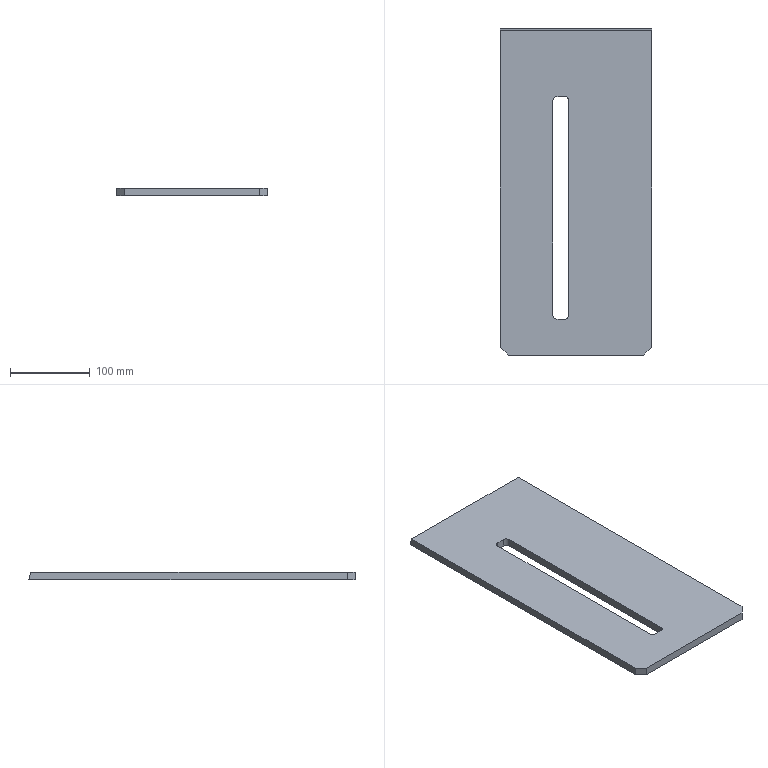Part | STEP file | 001-003-Shaft storage cylinder mounting plate | 1 solid | 16 faces | box 190 x 410.5 x 10 mm | volume 720796 mm3 | plane 12 | cylinder 4 | commonest cylinder face diameters 10 x4
STEP:
#1=CARTESIAN_POINT('',(0.,0.,0.));
#2=DIRECTION('',(0.,0.,1.));
#3=DIRECTION('',(1.,0.,0.));
#4=AXIS2_PLACEMENT_3D('',#1,#2,#3);
#5=CARTESIAN_POINT('',(95.,-195.25,10.));
#6=VERTEX_POINT('',#5);
#7=CARTESIAN_POINT('',(95.,202.757,10.));
#8=VERTEX_POINT('',#7);
#9=CARTESIAN_POINT('',(95.,-205.25,10.));
#10=DIRECTION('',(0.,1.,0.));
#11=VECTOR('',#10,1.);
#12=LINE('',#9,#11);
#13=CARTESIAN_POINT('',(95.,-205.25,10.));
#14=DIRECTION('',(-1.,0.,0.));
#15=DIRECTION('',(0.,0.,1.));
#16=AXIS2_PLACEMENT_3D('',#13,#14,#15);
#17=PLANE('',#16);
#18=CARTESIAN_POINT('',(0.,0.));
#19=DIRECTION('',(0.,1.));
#20=VECTOR('',#19,1.);
#21=LINE('',#18,#20);
#22=(GEOMETRIC_REPRESENTATION_CONTEXT(2)PARAMETRIC_REPRESENTATION_CONTEXT()REPRESENTATION_CONTEXT('',''));
#23=DEFINITIONAL_REPRESENTATION('',(#21),#22);
#24=PCURVE('',#17,#23);
#25=CARTESIAN_POINT('',(0.,0.,10.));
#26=DIRECTION('',(0.,0.,-1.));
#27=DIRECTION('',(-1.,0.,0.));
#28=AXIS2_PLACEMENT_3D('',#25,#26,#27);
#29=PLANE('',#28);
#30=CARTESIAN_POINT('',(-95.,-205.25));
#31=DIRECTION('',(0.,1.));
#32=VECTOR('',#31,1.);
#33=LINE('',#30,#32);
#34=(GEOMETRIC_REPRESENTATION_CONTEXT(2)PARAMETRIC_REPRESENTATION_CONTEXT()REPRESENTATION_CONTEXT('',''));
#35=DEFINITIONAL_REPRESENTATION('',(#33),#34);
#36=PCURVE('',#29,#35);
#37=SURFACE_CURVE('',#12,(#24,#36),.PCURVE_S1.);
#38=EDGE_CURVE('',#6,#8,#37,.T.);
#39=ORIENTED_EDGE('',*,*,#38,.F.);
#40=CARTESIAN_POINT('',(95.,-195.25,0.));
#41=VERTEX_POINT('',#40);
#42=CARTESIAN_POINT('',(95.,-195.25,10.));
#43=DIRECTION('',(0.,0.,-1.));
#44=VECTOR('',#43,1.);
#45=LINE('',#42,#44);
#46=CARTESIAN_POINT('',(0.,10.));
#47=DIRECTION('',(-1.,0.));
#48=VECTOR('',#47,1.);
#49=LINE('',#46,#48);
#50=(GEOMETRIC_REPRESENTATION_CONTEXT(2)PARAMETRIC_REPRESENTATION_CONTEXT()REPRESENTATION_CONTEXT('',''));
#51=DEFINITIONAL_REPRESENTATION('',(#49),#50);
#52=PCURVE('',#17,#51);
#53=CARTESIAN_POINT('',(95.,-195.25,10.));
#54=DIRECTION('',(-0.7071,0.7071,0.));
#55=DIRECTION('',(0.,0.,-1.));
#56=AXIS2_PLACEMENT_3D('',#53,#54,#55);
#57=PLANE('',#56);
#58=CARTESIAN_POINT('',(0.,0.));
#59=DIRECTION('',(1.,0.));
#60=VECTOR('',#59,1.);
#61=LINE('',#58,#60);
#62=(GEOMETRIC_REPRESENTATION_CONTEXT(2)PARAMETRIC_REPRESENTATION_CONTEXT()REPRESENTATION_CONTEXT('',''));
#63=DEFINITIONAL_REPRESENTATION('',(#61),#62);
#64=PCURVE('',#57,#63);
#65=SURFACE_CURVE('',#45,(#52,#64),.PCURVE_S1.);
#66=EDGE_CURVE('',#6,#41,#65,.T.);
#67=ORIENTED_EDGE('',*,*,#66,.T.);
#68=CARTESIAN_POINT('',(95.,205.25,0.));
#69=VERTEX_POINT('',#68);
#70=CARTESIAN_POINT('',(95.,-205.25,0.));
#71=DIRECTION('',(0.,1.,0.));
#72=VECTOR('',#71,1.);
#73=LINE('',#70,#72);
#74=CARTESIAN_POINT('',(-10.,0.));
#75=DIRECTION('',(0.,1.));
#76=VECTOR('',#75,1.);
#77=LINE('',#74,#76);
#78=(GEOMETRIC_REPRESENTATION_CONTEXT(2)PARAMETRIC_REPRESENTATION_CONTEXT()REPRESENTATION_CONTEXT('',''));
#79=DEFINITIONAL_REPRESENTATION('',(#77),#78);
#80=PCURVE('',#17,#79);
#81=CARTESIAN_POINT('',(0.,0.,0.));
#82=DIRECTION('',(0.,0.,-1.));
#83=DIRECTION('',(-1.,0.,0.));
#84=AXIS2_PLACEMENT_3D('',#81,#82,#83);
#85=PLANE('',#84);
#86=CARTESIAN_POINT('',(-95.,-205.25));
#87=DIRECTION('',(0.,1.));
#88=VECTOR('',#87,1.);
#89=LINE('',#86,#88);
#90=(GEOMETRIC_REPRESENTATION_CONTEXT(2)PARAMETRIC_REPRESENTATION_CONTEXT()REPRESENTATION_CONTEXT('',''));
#91=DEFINITIONAL_REPRESENTATION('',(#89),#90);
#92=PCURVE('',#85,#91);
#93=SURFACE_CURVE('',#73,(#80,#92),.PCURVE_S1.);
#94=EDGE_CURVE('',#41,#69,#93,.T.);
#95=ORIENTED_EDGE('',*,*,#94,.T.);
#96=CARTESIAN_POINT('',(95.,205.25,0.));
#97=DIRECTION('',(0.,0.2419,-0.9703));
#98=VECTOR('',#97,1.);
#99=LINE('',#96,#98);
#100=CARTESIAN_POINT('',(-10.,410.5));
#101=DIRECTION('',(-0.9703,0.2419));
#102=VECTOR('',#101,1.);
#103=LINE('',#100,#102);
#104=(GEOMETRIC_REPRESENTATION_CONTEXT(2)PARAMETRIC_REPRESENTATION_CONTEXT()REPRESENTATION_CONTEXT('',''));
#105=DEFINITIONAL_REPRESENTATION('',(#103),#104);
#106=PCURVE('',#17,#105);
#107=CARTESIAN_POINT('',(-95.,205.25,0.));
#108=DIRECTION('',(0.,-0.9703,-0.2419));
#109=DIRECTION('',(0.,0.2419,-0.9703));
#110=AXIS2_PLACEMENT_3D('',#107,#108,#109);
#111=PLANE('',#110);
#112=CARTESIAN_POINT('',(0.,190.));
#113=DIRECTION('',(1.,0.));
#114=VECTOR('',#113,1.);
#115=LINE('',#112,#114);
#116=(GEOMETRIC_REPRESENTATION_CONTEXT(2)PARAMETRIC_REPRESENTATION_CONTEXT()REPRESENTATION_CONTEXT('',''));
#117=DEFINITIONAL_REPRESENTATION('',(#115),#116);
#118=PCURVE('',#111,#117);
#119=SURFACE_CURVE('',#99,(#106,#118),.PCURVE_S1.);
#120=EDGE_CURVE('',#8,#69,#119,.T.);
#121=ORIENTED_EDGE('',*,*,#120,.F.);
#122=EDGE_LOOP('',(#39,#67,#95,#121));
#123=FACE_BOUND('',#122,.T.);
#124=ADVANCED_FACE('',(#123),#17,.F.);
#125=CARTESIAN_POINT('',(-95.,205.25,0.));
#126=VERTEX_POINT('',#125);
#127=CARTESIAN_POINT('',(-95.,-195.25,0.));
#128=VERTEX_POINT('',#127);
#129=CARTESIAN_POINT('',(-95.,-205.25,0.));
#130=DIRECTION('',(0.,-1.,0.));
#131=VECTOR('',#130,1.);
#132=LINE('',#129,#131);
#133=CARTESIAN_POINT('',(-95.,-205.25,10.));
#134=DIRECTION('',(1.,0.,0.));
#135=DIRECTION('',(0.,0.,-1.));
#136=AXIS2_PLACEMENT_3D('',#133,#134,#135);
#137=PLANE('',#136);
#138=CARTESIAN_POINT('',(10.,0.));
#139=DIRECTION('',(0.,-1.));
#140=VECTOR('',#139,1.);
#141=LINE('',#138,#140);
#142=(GEOMETRIC_REPRESENTATION_CONTEXT(2)PARAMETRIC_REPRESENTATION_CONTEXT()REPRESENTATION_CONTEXT('',''));
#143=DEFINITIONAL_REPRESENTATION('',(#141),#142);
#144=PCURVE('',#137,#143);
#145=CARTESIAN_POINT('',(95.,-205.25));
#146=DIRECTION('',(0.,-1.));
#147=VECTOR('',#146,1.);
#148=LINE('',#145,#147);
#149=(GEOMETRIC_REPRESENTATION_CONTEXT(2)PARAMETRIC_REPRESENTATION_CONTEXT()REPRESENTATION_CONTEXT('',''));
#150=DEFINITIONAL_REPRESENTATION('',(#148),#149);
#151=PCURVE('',#85,#150);
#152=SURFACE_CURVE('',#132,(#144,#151),.PCURVE_S1.);
#153=EDGE_CURVE('',#126,#128,#152,.T.);
#154=ORIENTED_EDGE('',*,*,#153,.T.);
#155=CARTESIAN_POINT('',(-95.,-195.25,10.));
#156=VERTEX_POINT('',#155);
#157=CARTESIAN_POINT('',(-95.,-195.25,10.));
#158=DIRECTION('',(0.,0.,1.));
#159=VECTOR('',#158,1.);
#160=LINE('',#157,#159);
#161=CARTESIAN_POINT('',(0.,10.));
#162=DIRECTION('',(-1.,0.));
#163=VECTOR('',#162,1.);
#164=LINE('',#161,#163);
#165=(GEOMETRIC_REPRESENTATION_CONTEXT(2)PARAMETRIC_REPRESENTATION_CONTEXT()REPRESENTATION_CONTEXT('',''));
#166=DEFINITIONAL_REPRESENTATION('',(#164),#165);
#167=PCURVE('',#137,#166);
#168=CARTESIAN_POINT('',(-85.,-205.25,10.));
#169=DIRECTION('',(0.7071,0.7071,0.));
#170=DIRECTION('',(0.,0.,-1.));
#171=AXIS2_PLACEMENT_3D('',#168,#169,#170);
#172=PLANE('',#171);
#173=CARTESIAN_POINT('',(0.,14.142));
#174=DIRECTION('',(-1.,0.));
#175=VECTOR('',#174,1.);
#176=LINE('',#173,#175);
#177=(GEOMETRIC_REPRESENTATION_CONTEXT(2)PARAMETRIC_REPRESENTATION_CONTEXT()REPRESENTATION_CONTEXT('',''));
#178=DEFINITIONAL_REPRESENTATION('',(#176),#177);
#179=PCURVE('',#172,#178);
#180=SURFACE_CURVE('',#160,(#167,#179),.PCURVE_S1.);
#181=EDGE_CURVE('',#128,#156,#180,.T.);
#182=ORIENTED_EDGE('',*,*,#181,.T.);
#183=CARTESIAN_POINT('',(-95.,202.757,10.));
#184=VERTEX_POINT('',#183);
#185=CARTESIAN_POINT('',(-95.,-205.25,10.));
#186=DIRECTION('',(0.,-1.,0.));
#187=VECTOR('',#186,1.);
#188=LINE('',#185,#187);
#189=CARTESIAN_POINT('',(0.,0.));
#190=DIRECTION('',(0.,-1.));
#191=VECTOR('',#190,1.);
#192=LINE('',#189,#191);
#193=(GEOMETRIC_REPRESENTATION_CONTEXT(2)PARAMETRIC_REPRESENTATION_CONTEXT()REPRESENTATION_CONTEXT('',''));
#194=DEFINITIONAL_REPRESENTATION('',(#192),#193);
#195=PCURVE('',#137,#194);
#196=CARTESIAN_POINT('',(95.,-205.25));
#197=DIRECTION('',(0.,-1.));
#198=VECTOR('',#197,1.);
#199=LINE('',#196,#198);
#200=(GEOMETRIC_REPRESENTATION_CONTEXT(2)PARAMETRIC_REPRESENTATION_CONTEXT()REPRESENTATION_CONTEXT('',''));
#201=DEFINITIONAL_REPRESENTATION('',(#199),#200);
#202=PCURVE('',#29,#201);
#203=SURFACE_CURVE('',#188,(#195,#202),.PCURVE_S1.);
#204=EDGE_CURVE('',#184,#156,#203,.T.);
#205=ORIENTED_EDGE('',*,*,#204,.F.);
#206=CARTESIAN_POINT('',(-95.,205.25,0.));
#207=DIRECTION('',(0.,0.2419,-0.9703));
#208=VECTOR('',#207,1.);
#209=LINE('',#206,#208);
#210=CARTESIAN_POINT('',(10.,410.5));
#211=DIRECTION('',(0.9703,0.2419));
#212=VECTOR('',#211,1.);
#213=LINE('',#210,#212);
#214=(GEOMETRIC_REPRESENTATION_CONTEXT(2)PARAMETRIC_REPRESENTATION_CONTEXT()REPRESENTATION_CONTEXT('',''));
#215=DEFINITIONAL_REPRESENTATION('',(#213),#214);
#216=PCURVE('',#137,#215);
#217=CARTESIAN_POINT('',(0.,0.));
#218=DIRECTION('',(1.,0.));
#219=VECTOR('',#218,1.);
#220=LINE('',#217,#219);
#221=(GEOMETRIC_REPRESENTATION_CONTEXT(2)PARAMETRIC_REPRESENTATION_CONTEXT()REPRESENTATION_CONTEXT('',''));
#222=DEFINITIONAL_REPRESENTATION('',(#220),#221);
#223=PCURVE('',#111,#222);
#224=SURFACE_CURVE('',#209,(#216,#223),.PCURVE_S1.);
#225=EDGE_CURVE('',#184,#126,#224,.T.);
#226=ORIENTED_EDGE('',*,*,#225,.T.);
#227=EDGE_LOOP('',(#154,#182,#205,#226));
#228=FACE_BOUND('',#227,.T.);
#229=ADVANCED_FACE('',(#228),#137,.F.);
#230=CARTESIAN_POINT('',(-85.,-205.25,0.));
#231=VERTEX_POINT('',#230);
#232=CARTESIAN_POINT('',(85.,-205.25,0.));
#233=VERTEX_POINT('',#232);
#234=CARTESIAN_POINT('',(-95.,-205.25,0.));
#235=DIRECTION('',(1.,0.,0.));
#236=VECTOR('',#235,1.);
#237=LINE('',#234,#236);
#238=CARTESIAN_POINT('',(-95.,-205.25,10.));
#239=DIRECTION('',(0.,1.,0.));
#240=DIRECTION('',(0.,0.,1.));
#241=AXIS2_PLACEMENT_3D('',#238,#239,#240);
#242=PLANE('',#241);
#243=CARTESIAN_POINT('',(-10.,0.));
#244=DIRECTION('',(0.,1.));
#245=VECTOR('',#244,1.);
#246=LINE('',#243,#245);
#247=(GEOMETRIC_REPRESENTATION_CONTEXT(2)PARAMETRIC_REPRESENTATION_CONTEXT()REPRESENTATION_CONTEXT('',''));
#248=DEFINITIONAL_REPRESENTATION('',(#246),#247);
#249=PCURVE('',#242,#248);
#250=CARTESIAN_POINT('',(95.,-205.25));
#251=DIRECTION('',(-1.,0.));
#252=VECTOR('',#251,1.);
#253=LINE('',#250,#252);
#254=(GEOMETRIC_REPRESENTATION_CONTEXT(2)PARAMETRIC_REPRESENTATION_CONTEXT()REPRESENTATION_CONTEXT('',''));
#255=DEFINITIONAL_REPRESENTATION('',(#253),#254);
#256=PCURVE('',#85,#255);
#257=SURFACE_CURVE('',#237,(#249,#256),.PCURVE_S1.);
#258=EDGE_CURVE('',#231,#233,#257,.T.);
#259=ORIENTED_EDGE('',*,*,#258,.T.);
#260=CARTESIAN_POINT('',(85.,-205.25,10.));
#261=VERTEX_POINT('',#260);
#262=CARTESIAN_POINT('',(85.,-205.25,10.));
#263=DIRECTION('',(0.,0.,1.));
#264=VECTOR('',#263,1.);
#265=LINE('',#262,#264);
#266=CARTESIAN_POINT('',(0.,180.));
#267=DIRECTION('',(1.,0.));
#268=VECTOR('',#267,1.);
#269=LINE('',#266,#268);
#270=(GEOMETRIC_REPRESENTATION_CONTEXT(2)PARAMETRIC_REPRESENTATION_CONTEXT()REPRESENTATION_CONTEXT('',''));
#271=DEFINITIONAL_REPRESENTATION('',(#269),#270);
#272=PCURVE('',#242,#271);
#273=CARTESIAN_POINT('',(0.,14.142));
#274=DIRECTION('',(-1.,0.));
#275=VECTOR('',#274,1.);
#276=LINE('',#273,#275);
#277=(GEOMETRIC_REPRESENTATION_CONTEXT(2)PARAMETRIC_REPRESENTATION_CONTEXT()REPRESENTATION_CONTEXT('',''));
#278=DEFINITIONAL_REPRESENTATION('',(#276),#277);
#279=PCURVE('',#57,#278);
#280=SURFACE_CURVE('',#265,(#272,#279),.PCURVE_S1.);
#281=EDGE_CURVE('',#233,#261,#280,.T.);
#282=ORIENTED_EDGE('',*,*,#281,.T.);
#283=CARTESIAN_POINT('',(-85.,-205.25,10.));
#284=VERTEX_POINT('',#283);
#285=CARTESIAN_POINT('',(-95.,-205.25,10.));
#286=DIRECTION('',(1.,0.,0.));
#287=VECTOR('',#286,1.);
#288=LINE('',#285,#287);
#289=CARTESIAN_POINT('',(0.,0.));
#290=DIRECTION('',(0.,1.));
#291=VECTOR('',#290,1.);
#292=LINE('',#289,#291);
#293=(GEOMETRIC_REPRESENTATION_CONTEXT(2)PARAMETRIC_REPRESENTATION_CONTEXT()REPRESENTATION_CONTEXT('',''));
#294=DEFINITIONAL_REPRESENTATION('',(#292),#293);
#295=PCURVE('',#242,#294);
#296=CARTESIAN_POINT('',(95.,-205.25));
#297=DIRECTION('',(-1.,0.));
#298=VECTOR('',#297,1.);
#299=LINE('',#296,#298);
#300=(GEOMETRIC_REPRESENTATION_CONTEXT(2)PARAMETRIC_REPRESENTATION_CONTEXT()REPRESENTATION_CONTEXT('',''));
#301=DEFINITIONAL_REPRESENTATION('',(#299),#300);
#302=PCURVE('',#29,#301);
#303=SURFACE_CURVE('',#288,(#295,#302),.PCURVE_S1.);
#304=EDGE_CURVE('',#284,#261,#303,.T.);
#305=ORIENTED_EDGE('',*,*,#304,.F.);
#306=CARTESIAN_POINT('',(-85.,-205.25,10.));
#307=DIRECTION('',(0.,0.,-1.));
#308=VECTOR('',#307,1.);
#309=LINE('',#306,#308);
#310=CARTESIAN_POINT('',(0.,10.));
#311=DIRECTION('',(-1.,0.));
#312=VECTOR('',#311,1.);
#313=LINE('',#310,#312);
#314=(GEOMETRIC_REPRESENTATION_CONTEXT(2)PARAMETRIC_REPRESENTATION_CONTEXT()REPRESENTATION_CONTEXT('',''));
#315=DEFINITIONAL_REPRESENTATION('',(#313),#314);
#316=PCURVE('',#242,#315);
#317=CARTESIAN_POINT('',(0.,0.));
#318=DIRECTION('',(1.,0.));
#319=VECTOR('',#318,1.);
#320=LINE('',#317,#319);
#321=(GEOMETRIC_REPRESENTATION_CONTEXT(2)PARAMETRIC_REPRESENTATION_CONTEXT()REPRESENTATION_CONTEXT('',''));
#322=DEFINITIONAL_REPRESENTATION('',(#320),#321);
#323=PCURVE('',#172,#322);
#324=SURFACE_CURVE('',#309,(#316,#323),.PCURVE_S1.);
#325=EDGE_CURVE('',#284,#231,#324,.T.);
#326=ORIENTED_EDGE('',*,*,#325,.T.);
#327=EDGE_LOOP('',(#259,#282,#305,#326));
#328=FACE_BOUND('',#327,.T.);
#329=ADVANCED_FACE('',(#328),#242,.F.);
#330=CARTESIAN_POINT('',(-14.,120.,10.));
#331=VERTEX_POINT('',#330);
#332=CARTESIAN_POINT('',(-24.,120.,10.));
#333=VERTEX_POINT('',#332);
#334=CARTESIAN_POINT('',(-9.,120.,10.));
#335=DIRECTION('',(-1.,0.,0.));
#336=VECTOR('',#335,1.);
#337=LINE('',#334,#336);
#338=CARTESIAN_POINT('',(9.,120.));
#339=DIRECTION('',(1.,0.));
#340=VECTOR('',#339,1.);
#341=LINE('',#338,#340);
#342=(GEOMETRIC_REPRESENTATION_CONTEXT(2)PARAMETRIC_REPRESENTATION_CONTEXT()REPRESENTATION_CONTEXT('',''));
#343=DEFINITIONAL_REPRESENTATION('',(#341),#342);
#344=PCURVE('',#29,#343);
#345=CARTESIAN_POINT('',(-9.,120.,0.));
#346=DIRECTION('',(0.,1.,0.));
#347=DIRECTION('',(0.,0.,1.));
#348=AXIS2_PLACEMENT_3D('',#345,#346,#347);
#349=PLANE('',#348);
#350=CARTESIAN_POINT('',(10.,0.));
#351=DIRECTION('',(0.,-1.));
#352=VECTOR('',#351,1.);
#353=LINE('',#350,#352);
#354=(GEOMETRIC_REPRESENTATION_CONTEXT(2)PARAMETRIC_REPRESENTATION_CONTEXT()REPRESENTATION_CONTEXT('',''));
#355=DEFINITIONAL_REPRESENTATION('',(#353),#354);
#356=PCURVE('',#349,#355);
#357=SURFACE_CURVE('',#337,(#344,#356),.PCURVE_S1.);
#358=EDGE_CURVE('',#331,#333,#357,.T.);
#359=ORIENTED_EDGE('',*,*,#358,.F.);
#360=CARTESIAN_POINT('',(-9.,115.,10.));
#361=VERTEX_POINT('',#360);
#362=CARTESIAN_POINT('',(-14.,115.,10.));
#363=DIRECTION('',(0.,0.,-1.));
#364=DIRECTION('',(-1.,0.,0.));
#365=AXIS2_PLACEMENT_3D('',#362,#363,#364);
#366=CIRCLE('',#365,5.);
#367=CARTESIAN_POINT('',(14.,115.));
#368=DIRECTION('',(1.,0.));
#369=AXIS2_PLACEMENT_2D('',#367,#368);
#370=CIRCLE('',#369,5.);
#371=(GEOMETRIC_REPRESENTATION_CONTEXT(2)PARAMETRIC_REPRESENTATION_CONTEXT()REPRESENTATION_CONTEXT('',''));
#372=DEFINITIONAL_REPRESENTATION('',(#370),#371);
#373=PCURVE('',#29,#372);
#374=CARTESIAN_POINT('',(-14.,115.,0.));
#375=DIRECTION('',(0.,0.,-1.));
#376=DIRECTION('',(-1.,0.,0.));
#377=AXIS2_PLACEMENT_3D('',#374,#375,#376);
#378=CYLINDRICAL_SURFACE('',#377,5.);
#379=CARTESIAN_POINT('',(0.,-10.));
#380=DIRECTION('',(1.,0.));
#381=VECTOR('',#380,1.);
#382=LINE('',#379,#381);
#383=(GEOMETRIC_REPRESENTATION_CONTEXT(2)PARAMETRIC_REPRESENTATION_CONTEXT()REPRESENTATION_CONTEXT('',''));
#384=DEFINITIONAL_REPRESENTATION('',(#382),#383);
#385=PCURVE('',#378,#384);
#386=SURFACE_CURVE('',#366,(#373,#385),.PCURVE_S1.);
#387=EDGE_CURVE('',#331,#361,#386,.T.);
#388=ORIENTED_EDGE('',*,*,#387,.T.);
#389=CARTESIAN_POINT('',(-9.,-155.,10.));
#390=VERTEX_POINT('',#389);
#391=CARTESIAN_POINT('',(-9.,-160.,10.));
#392=DIRECTION('',(0.,1.,0.));
#393=VECTOR('',#392,1.);
#394=LINE('',#391,#393);
#395=CARTESIAN_POINT('',(9.,-160.));
#396=DIRECTION('',(0.,1.));
#397=VECTOR('',#396,1.);
#398=LINE('',#395,#397);
#399=(GEOMETRIC_REPRESENTATION_CONTEXT(2)PARAMETRIC_REPRESENTATION_CONTEXT()REPRESENTATION_CONTEXT('',''));
#400=DEFINITIONAL_REPRESENTATION('',(#398),#399);
#401=PCURVE('',#29,#400);
#402=CARTESIAN_POINT('',(-9.,-160.,0.));
#403=DIRECTION('',(1.,0.,0.));
#404=DIRECTION('',(0.,0.,-1.));
#405=AXIS2_PLACEMENT_3D('',#402,#403,#404);
#406=PLANE('',#405);
#407=CARTESIAN_POINT('',(-10.,0.));
#408=DIRECTION('',(0.,1.));
#409=VECTOR('',#408,1.);
#410=LINE('',#407,#409);
#411=(GEOMETRIC_REPRESENTATION_CONTEXT(2)PARAMETRIC_REPRESENTATION_CONTEXT()REPRESENTATION_CONTEXT('',''));
#412=DEFINITIONAL_REPRESENTATION('',(#410),#411);
#413=PCURVE('',#406,#412);
#414=SURFACE_CURVE('',#394,(#401,#413),.PCURVE_S1.);
#415=EDGE_CURVE('',#390,#361,#414,.T.);
#416=ORIENTED_EDGE('',*,*,#415,.F.);
#417=CARTESIAN_POINT('',(-14.,-160.,10.));
#418=VERTEX_POINT('',#417);
#419=CARTESIAN_POINT('',(-14.,-155.,10.));
#420=DIRECTION('',(0.,0.,-1.));
#421=DIRECTION('',(-1.,0.,0.));
#422=AXIS2_PLACEMENT_3D('',#419,#420,#421);
#423=CIRCLE('',#422,5.);
#424=CARTESIAN_POINT('',(14.,-155.));
#425=DIRECTION('',(1.,0.));
#426=AXIS2_PLACEMENT_2D('',#424,#425);
#427=CIRCLE('',#426,5.);
#428=(GEOMETRIC_REPRESENTATION_CONTEXT(2)PARAMETRIC_REPRESENTATION_CONTEXT()REPRESENTATION_CONTEXT('',''));
#429=DEFINITIONAL_REPRESENTATION('',(#427),#428);
#430=PCURVE('',#29,#429);
#431=CARTESIAN_POINT('',(-14.,-155.,0.));
#432=DIRECTION('',(0.,0.,-1.));
#433=DIRECTION('',(-1.,0.,0.));
#434=AXIS2_PLACEMENT_3D('',#431,#432,#433);
#435=CYLINDRICAL_SURFACE('',#434,5.);
#436=CARTESIAN_POINT('',(0.,-10.));
#437=DIRECTION('',(1.,0.));
#438=VECTOR('',#437,1.);
#439=LINE('',#436,#438);
#440=(GEOMETRIC_REPRESENTATION_CONTEXT(2)PARAMETRIC_REPRESENTATION_CONTEXT()REPRESENTATION_CONTEXT('',''));
#441=DEFINITIONAL_REPRESENTATION('',(#439),#440);
#442=PCURVE('',#435,#441);
#443=SURFACE_CURVE('',#423,(#430,#442),.PCURVE_S1.);
#444=EDGE_CURVE('',#390,#418,#443,.T.);
#445=ORIENTED_EDGE('',*,*,#444,.T.);
#446=CARTESIAN_POINT('',(-24.,-160.,10.));
#447=VERTEX_POINT('',#446);
#448=CARTESIAN_POINT('',(-9.,-160.,10.));
#449=DIRECTION('',(1.,0.,0.));
#450=VECTOR('',#449,1.);
#451=LINE('',#448,#450);
#452=CARTESIAN_POINT('',(9.,-160.));
#453=DIRECTION('',(-1.,0.));
#454=VECTOR('',#453,1.);
#455=LINE('',#452,#454);
#456=(GEOMETRIC_REPRESENTATION_CONTEXT(2)PARAMETRIC_REPRESENTATION_CONTEXT()REPRESENTATION_CONTEXT('',''));
#457=DEFINITIONAL_REPRESENTATION('',(#455),#456);
#458=PCURVE('',#29,#457);
#459=CARTESIAN_POINT('',(-9.,-160.,0.));
#460=DIRECTION('',(0.,-1.,0.));
#461=DIRECTION('',(1.,0.,0.));
#462=AXIS2_PLACEMENT_3D('',#459,#460,#461);
#463=PLANE('',#462);
#464=CARTESIAN_POINT('',(0.,10.));
#465=DIRECTION('',(1.,0.));
#466=VECTOR('',#465,1.);
#467=LINE('',#464,#466);
#468=(GEOMETRIC_REPRESENTATION_CONTEXT(2)PARAMETRIC_REPRESENTATION_CONTEXT()REPRESENTATION_CONTEXT('',''));
#469=DEFINITIONAL_REPRESENTATION('',(#467),#468);
#470=PCURVE('',#463,#469);
#471=SURFACE_CURVE('',#451,(#458,#470),.PCURVE_S1.);
#472=EDGE_CURVE('',#447,#418,#471,.T.);
#473=ORIENTED_EDGE('',*,*,#472,.F.);
#474=CARTESIAN_POINT('',(-29.,-155.,10.));
#475=VERTEX_POINT('',#474);
#476=CARTESIAN_POINT('',(-24.,-155.,10.));
#477=DIRECTION('',(0.,0.,-1.));
#478=DIRECTION('',(-1.,0.,0.));
#479=AXIS2_PLACEMENT_3D('',#476,#477,#478);
#480=CIRCLE('',#479,5.);
#481=CARTESIAN_POINT('',(24.,-155.));
#482=DIRECTION('',(1.,0.));
#483=AXIS2_PLACEMENT_2D('',#481,#482);
#484=CIRCLE('',#483,5.);
#485=(GEOMETRIC_REPRESENTATION_CONTEXT(2)PARAMETRIC_REPRESENTATION_CONTEXT()REPRESENTATION_CONTEXT('',''));
#486=DEFINITIONAL_REPRESENTATION('',(#484),#485);
#487=PCURVE('',#29,#486);
#488=CARTESIAN_POINT('',(-24.,-155.,0.));
#489=DIRECTION('',(0.,0.,-1.));
#490=DIRECTION('',(-1.,0.,0.));
#491=AXIS2_PLACEMENT_3D('',#488,#489,#490);
#492=CYLINDRICAL_SURFACE('',#491,5.);
#493=CARTESIAN_POINT('',(0.,-10.));
#494=DIRECTION('',(1.,0.));
#495=VECTOR('',#494,1.);
#496=LINE('',#493,#495);
#497=(GEOMETRIC_REPRESENTATION_CONTEXT(2)PARAMETRIC_REPRESENTATION_CONTEXT()REPRESENTATION_CONTEXT('',''));
#498=DEFINITIONAL_REPRESENTATION('',(#496),#497);
#499=PCURVE('',#492,#498);
#500=SURFACE_CURVE('',#480,(#487,#499),.PCURVE_S1.);
#501=EDGE_CURVE('',#447,#475,#500,.T.);
#502=ORIENTED_EDGE('',*,*,#501,.T.);
#503=CARTESIAN_POINT('',(-29.,115.,10.));
#504=VERTEX_POINT('',#503);
#505=CARTESIAN_POINT('',(-29.,-160.,10.));
#506=DIRECTION('',(0.,-1.,0.));
#507=VECTOR('',#506,1.);
#508=LINE('',#505,#507);
#509=CARTESIAN_POINT('',(29.,-160.));
#510=DIRECTION('',(0.,-1.));
#511=VECTOR('',#510,1.);
#512=LINE('',#509,#511);
#513=(GEOMETRIC_REPRESENTATION_CONTEXT(2)PARAMETRIC_REPRESENTATION_CONTEXT()REPRESENTATION_CONTEXT('',''));
#514=DEFINITIONAL_REPRESENTATION('',(#512),#513);
#515=PCURVE('',#29,#514);
#516=CARTESIAN_POINT('',(-29.,-160.,0.));
#517=DIRECTION('',(-1.,0.,0.));
#518=DIRECTION('',(0.,-1.,0.));
#519=AXIS2_PLACEMENT_3D('',#516,#517,#518);
#520=PLANE('',#519);
#521=CARTESIAN_POINT('',(0.,10.));
#522=DIRECTION('',(1.,0.));
#523=VECTOR('',#522,1.);
#524=LINE('',#521,#523);
#525=(GEOMETRIC_REPRESENTATION_CONTEXT(2)PARAMETRIC_REPRESENTATION_CONTEXT()REPRESENTATION_CONTEXT('',''));
#526=DEFINITIONAL_REPRESENTATION('',(#524),#525);
#527=PCURVE('',#520,#526);
#528=SURFACE_CURVE('',#508,(#515,#527),.PCURVE_S1.);
#529=EDGE_CURVE('',#504,#475,#528,.T.);
#530=ORIENTED_EDGE('',*,*,#529,.F.);
#531=CARTESIAN_POINT('',(-24.,115.,10.));
#532=DIRECTION('',(0.,0.,-1.));
#533=DIRECTION('',(-1.,0.,0.));
#534=AXIS2_PLACEMENT_3D('',#531,#532,#533);
#535=CIRCLE('',#534,5.);
#536=CARTESIAN_POINT('',(24.,115.));
#537=DIRECTION('',(1.,0.));
#538=AXIS2_PLACEMENT_2D('',#536,#537);
#539=CIRCLE('',#538,5.);
#540=(GEOMETRIC_REPRESENTATION_CONTEXT(2)PARAMETRIC_REPRESENTATION_CONTEXT()REPRESENTATION_CONTEXT('',''));
#541=DEFINITIONAL_REPRESENTATION('',(#539),#540);
#542=PCURVE('',#29,#541);
#543=CARTESIAN_POINT('',(-24.,115.,0.));
#544=DIRECTION('',(0.,0.,-1.));
#545=DIRECTION('',(-1.,0.,0.));
#546=AXIS2_PLACEMENT_3D('',#543,#544,#545);
#547=CYLINDRICAL_SURFACE('',#546,5.);
#548=CARTESIAN_POINT('',(0.,-10.));
#549=DIRECTION('',(1.,0.));
#550=VECTOR('',#549,1.);
#551=LINE('',#548,#550);
#552=(GEOMETRIC_REPRESENTATION_CONTEXT(2)PARAMETRIC_REPRESENTATION_CONTEXT()REPRESENTATION_CONTEXT('',''));
#553=DEFINITIONAL_REPRESENTATION('',(#551),#552);
#554=PCURVE('',#547,#553);
#555=SURFACE_CURVE('',#535,(#542,#554),.PCURVE_S1.);
#556=EDGE_CURVE('',#504,#333,#555,.T.);
#557=ORIENTED_EDGE('',*,*,#556,.T.);
#558=EDGE_LOOP('',(#359,#388,#416,#445,#473,#502,#530,#557));
#559=FACE_BOUND('',#558,.T.);
#560=ORIENTED_EDGE('',*,*,#304,.T.);
#561=CARTESIAN_POINT('',(95.,-195.25,10.));
#562=DIRECTION('',(0.7071,0.7071,0.));
#563=VECTOR('',#562,1.);
#564=LINE('',#561,#563);
#565=CARTESIAN_POINT('',(-95.,-195.25));
#566=DIRECTION('',(-0.7071,0.7071));
#567=VECTOR('',#566,1.);
#568=LINE('',#565,#567);
#569=(GEOMETRIC_REPRESENTATION_CONTEXT(2)PARAMETRIC_REPRESENTATION_CONTEXT()REPRESENTATION_CONTEXT('',''));
#570=DEFINITIONAL_REPRESENTATION('',(#568),#569);
#571=PCURVE('',#29,#570);
#572=CARTESIAN_POINT('',(0.,0.));
#573=DIRECTION('',(0.,-1.));
#574=VECTOR('',#573,1.);
#575=LINE('',#572,#574);
#576=(GEOMETRIC_REPRESENTATION_CONTEXT(2)PARAMETRIC_REPRESENTATION_CONTEXT()REPRESENTATION_CONTEXT('',''));
#577=DEFINITIONAL_REPRESENTATION('',(#575),#576);
#578=PCURVE('',#57,#577);
#579=SURFACE_CURVE('',#564,(#571,#578),.PCURVE_S1.);
#580=EDGE_CURVE('',#261,#6,#579,.T.);
#581=ORIENTED_EDGE('',*,*,#580,.T.);
#582=ORIENTED_EDGE('',*,*,#38,.T.);
#583=CARTESIAN_POINT('',(-95.,202.757,10.));
#584=DIRECTION('',(1.,0.,0.));
#585=VECTOR('',#584,1.);
#586=LINE('',#583,#585);
#587=CARTESIAN_POINT('',(95.,202.757));
#588=DIRECTION('',(-1.,0.));
#589=VECTOR('',#588,1.);
#590=LINE('',#587,#589);
#591=(GEOMETRIC_REPRESENTATION_CONTEXT(2)PARAMETRIC_REPRESENTATION_CONTEXT()REPRESENTATION_CONTEXT('',''));
#592=DEFINITIONAL_REPRESENTATION('',(#590),#591);
#593=PCURVE('',#29,#592);
#594=CARTESIAN_POINT('',(-10.306,0.));
#595=DIRECTION('',(0.,1.));
#596=VECTOR('',#595,1.);
#597=LINE('',#594,#596);
#598=(GEOMETRIC_REPRESENTATION_CONTEXT(2)PARAMETRIC_REPRESENTATION_CONTEXT()REPRESENTATION_CONTEXT('',''));
#599=DEFINITIONAL_REPRESENTATION('',(#597),#598);
#600=PCURVE('',#111,#599);
#601=SURFACE_CURVE('',#586,(#593,#600),.PCURVE_S1.);
#602=EDGE_CURVE('',#184,#8,#601,.T.);
#603=ORIENTED_EDGE('',*,*,#602,.F.);
#604=ORIENTED_EDGE('',*,*,#204,.T.);
#605=CARTESIAN_POINT('',(-85.,-205.25,10.));
#606=DIRECTION('',(0.7071,-0.7071,0.));
#607=VECTOR('',#606,1.);
#608=LINE('',#605,#607);
#609=CARTESIAN_POINT('',(85.,-205.25));
#610=DIRECTION('',(-0.7071,-0.7071));
#611=VECTOR('',#610,1.);
#612=LINE('',#609,#611);
#613=(GEOMETRIC_REPRESENTATION_CONTEXT(2)PARAMETRIC_REPRESENTATION_CONTEXT()REPRESENTATION_CONTEXT('',''));
#614=DEFINITIONAL_REPRESENTATION('',(#612),#613);
#615=PCURVE('',#29,#614);
#616=CARTESIAN_POINT('',(0.,0.));
#617=DIRECTION('',(0.,-1.));
#618=VECTOR('',#617,1.);
#619=LINE('',#616,#618);
#620=(GEOMETRIC_REPRESENTATION_CONTEXT(2)PARAMETRIC_REPRESENTATION_CONTEXT()REPRESENTATION_CONTEXT('',''));
#621=DEFINITIONAL_REPRESENTATION('',(#619),#620);
#622=PCURVE('',#172,#621);
#623=SURFACE_CURVE('',#608,(#615,#622),.PCURVE_S1.);
#624=EDGE_CURVE('',#156,#284,#623,.T.);
#625=ORIENTED_EDGE('',*,*,#624,.T.);
#626=EDGE_LOOP('',(#560,#581,#582,#603,#604,#625));
#627=FACE_BOUND('',#626,.T.);
#628=ADVANCED_FACE('',(#559,#627),#29,.F.);
#629=CARTESIAN_POINT('',(-24.,-160.,0.));
#630=VERTEX_POINT('',#629);
#631=CARTESIAN_POINT('',(-14.,-160.,0.));
#632=VERTEX_POINT('',#631);
#633=CARTESIAN_POINT('',(-9.,-160.,0.));
#634=DIRECTION('',(1.,0.,0.));
#635=VECTOR('',#634,1.);
#636=LINE('',#633,#635);
#637=CARTESIAN_POINT('',(9.,-160.));
#638=DIRECTION('',(-1.,0.));
#639=VECTOR('',#638,1.);
#640=LINE('',#637,#639);
#641=(GEOMETRIC_REPRESENTATION_CONTEXT(2)PARAMETRIC_REPRESENTATION_CONTEXT()REPRESENTATION_CONTEXT('',''));
#642=DEFINITIONAL_REPRESENTATION('',(#640),#641);
#643=PCURVE('',#85,#642);
#644=CARTESIAN_POINT('',(0.,0.));
#645=DIRECTION('',(1.,0.));
#646=VECTOR('',#645,1.);
#647=LINE('',#644,#646);
#648=(GEOMETRIC_REPRESENTATION_CONTEXT(2)PARAMETRIC_REPRESENTATION_CONTEXT()REPRESENTATION_CONTEXT('',''));
#649=DEFINITIONAL_REPRESENTATION('',(#647),#648);
#650=PCURVE('',#463,#649);
#651=SURFACE_CURVE('',#636,(#643,#650),.PCURVE_S1.);
#652=EDGE_CURVE('',#630,#632,#651,.T.);
#653=ORIENTED_EDGE('',*,*,#652,.T.);
#654=CARTESIAN_POINT('',(-9.,-155.,0.));
#655=VERTEX_POINT('',#654);
#656=CARTESIAN_POINT('',(-14.,-155.,0.));
#657=DIRECTION('',(0.,0.,1.));
#658=DIRECTION('',(-1.,0.,0.));
#659=AXIS2_PLACEMENT_3D('',#656,#657,#658);
#660=CIRCLE('',#659,5.);
#661=CARTESIAN_POINT('',(19.,-155.));
#662=CARTESIAN_POINT('',(19.,-163.66));
#663=CARTESIAN_POINT('',(11.5,-159.33));
#664=CARTESIAN_POINT('',(4.,-155.));
#665=CARTESIAN_POINT('',(11.5,-150.67));
#666=CARTESIAN_POINT('',(19.,-146.34));
#667=CARTESIAN_POINT('',(19.,-155.));
#668=(BOUNDED_CURVE()B_SPLINE_CURVE(2,(#661,#662,#663,#664,#665,#666,#667),.UNSPECIFIED.,.T.,.F.)B_SPLINE_CURVE_WITH_KNOTS((1,2,2,2,2,1),(-2.094,0.,2.094,4.189,6.283,8.378),.UNSPECIFIED.)CURVE()GEOMETRIC_REPRESENTATION_ITEM()RATIONAL_B_SPLINE_CURVE((1.,0.5,1.,0.5,1.,0.5,1.))REPRESENTATION_ITEM(''));
#669=(GEOMETRIC_REPRESENTATION_CONTEXT(2)PARAMETRIC_REPRESENTATION_CONTEXT()REPRESENTATION_CONTEXT('',''));
#670=DEFINITIONAL_REPRESENTATION('',(#668),#669);
#671=PCURVE('',#85,#670);
#672=CARTESIAN_POINT('',(6.283,0.));
#673=DIRECTION('',(-1.,0.));
#674=VECTOR('',#673,1.);
#675=LINE('',#672,#674);
#676=(GEOMETRIC_REPRESENTATION_CONTEXT(2)PARAMETRIC_REPRESENTATION_CONTEXT()REPRESENTATION_CONTEXT('',''));
#677=DEFINITIONAL_REPRESENTATION('',(#675),#676);
#678=PCURVE('',#435,#677);
#679=SURFACE_CURVE('',#660,(#671,#678),.PCURVE_S1.);
#680=EDGE_CURVE('',#632,#655,#679,.T.);
#681=ORIENTED_EDGE('',*,*,#680,.T.);
#682=CARTESIAN_POINT('',(-9.,115.,0.));
#683=VERTEX_POINT('',#682);
#684=CARTESIAN_POINT('',(-9.,-160.,0.));
#685=DIRECTION('',(0.,1.,0.));
#686=VECTOR('',#685,1.);
#687=LINE('',#684,#686);
#688=CARTESIAN_POINT('',(9.,-160.));
#689=DIRECTION('',(0.,1.));
#690=VECTOR('',#689,1.);
#691=LINE('',#688,#690);
#692=(GEOMETRIC_REPRESENTATION_CONTEXT(2)PARAMETRIC_REPRESENTATION_CONTEXT()REPRESENTATION_CONTEXT('',''));
#693=DEFINITIONAL_REPRESENTATION('',(#691),#692);
#694=PCURVE('',#85,#693);
#695=CARTESIAN_POINT('',(0.,0.));
#696=DIRECTION('',(0.,1.));
#697=VECTOR('',#696,1.);
#698=LINE('',#695,#697);
#699=(GEOMETRIC_REPRESENTATION_CONTEXT(2)PARAMETRIC_REPRESENTATION_CONTEXT()REPRESENTATION_CONTEXT('',''));
#700=DEFINITIONAL_REPRESENTATION('',(#698),#699);
#701=PCURVE('',#406,#700);
#702=SURFACE_CURVE('',#687,(#694,#701),.PCURVE_S1.);
#703=EDGE_CURVE('',#655,#683,#702,.T.);
#704=ORIENTED_EDGE('',*,*,#703,.T.);
#705=CARTESIAN_POINT('',(-14.,120.,0.));
#706=VERTEX_POINT('',#705);
#707=CARTESIAN_POINT('',(-14.,115.,0.));
#708=DIRECTION('',(0.,0.,1.));
#709=DIRECTION('',(-1.,0.,0.));
#710=AXIS2_PLACEMENT_3D('',#707,#708,#709);
#711=CIRCLE('',#710,5.);
#712=CARTESIAN_POINT('',(19.,115.));
#713=CARTESIAN_POINT('',(19.,106.34));
#714=CARTESIAN_POINT('',(11.5,110.67));
#715=CARTESIAN_POINT('',(4.,115.));
#716=CARTESIAN_POINT('',(11.5,119.33));
#717=CARTESIAN_POINT('',(19.,123.66));
#718=CARTESIAN_POINT('',(19.,115.));
#719=(BOUNDED_CURVE()B_SPLINE_CURVE(2,(#712,#713,#714,#715,#716,#717,#718),.UNSPECIFIED.,.T.,.F.)B_SPLINE_CURVE_WITH_KNOTS((1,2,2,2,2,1),(-2.094,0.,2.094,4.189,6.283,8.378),.UNSPECIFIED.)CURVE()GEOMETRIC_REPRESENTATION_ITEM()RATIONAL_B_SPLINE_CURVE((1.,0.5,1.,0.5,1.,0.5,1.))REPRESENTATION_ITEM(''));
#720=(GEOMETRIC_REPRESENTATION_CONTEXT(2)PARAMETRIC_REPRESENTATION_CONTEXT()REPRESENTATION_CONTEXT('',''));
#721=DEFINITIONAL_REPRESENTATION('',(#719),#720);
#722=PCURVE('',#85,#721);
#723=CARTESIAN_POINT('',(6.283,0.));
#724=DIRECTION('',(-1.,0.));
#725=VECTOR('',#724,1.);
#726=LINE('',#723,#725);
#727=(GEOMETRIC_REPRESENTATION_CONTEXT(2)PARAMETRIC_REPRESENTATION_CONTEXT()REPRESENTATION_CONTEXT('',''));
#728=DEFINITIONAL_REPRESENTATION('',(#726),#727);
#729=PCURVE('',#378,#728);
#730=SURFACE_CURVE('',#711,(#722,#729),.PCURVE_S1.);
#731=EDGE_CURVE('',#683,#706,#730,.T.);
#732=ORIENTED_EDGE('',*,*,#731,.T.);
#733=CARTESIAN_POINT('',(-24.,120.,0.));
#734=VERTEX_POINT('',#733);
#735=CARTESIAN_POINT('',(-9.,120.,0.));
#736=DIRECTION('',(-1.,0.,0.));
#737=VECTOR('',#736,1.);
#738=LINE('',#735,#737);
#739=CARTESIAN_POINT('',(9.,120.));
#740=DIRECTION('',(1.,0.));
#741=VECTOR('',#740,1.);
#742=LINE('',#739,#741);
#743=(GEOMETRIC_REPRESENTATION_CONTEXT(2)PARAMETRIC_REPRESENTATION_CONTEXT()REPRESENTATION_CONTEXT('',''));
#744=DEFINITIONAL_REPRESENTATION('',(#742),#743);
#745=PCURVE('',#85,#744);
#746=CARTESIAN_POINT('',(0.,0.));
#747=DIRECTION('',(0.,-1.));
#748=VECTOR('',#747,1.);
#749=LINE('',#746,#748);
#750=(GEOMETRIC_REPRESENTATION_CONTEXT(2)PARAMETRIC_REPRESENTATION_CONTEXT()REPRESENTATION_CONTEXT('',''));
#751=DEFINITIONAL_REPRESENTATION('',(#749),#750);
#752=PCURVE('',#349,#751);
#753=SURFACE_CURVE('',#738,(#745,#752),.PCURVE_S1.);
#754=EDGE_CURVE('',#706,#734,#753,.T.);
#755=ORIENTED_EDGE('',*,*,#754,.T.);
#756=CARTESIAN_POINT('',(-29.,115.,0.));
#757=VERTEX_POINT('',#756);
#758=CARTESIAN_POINT('',(-24.,115.,0.));
#759=DIRECTION('',(0.,0.,1.));
#760=DIRECTION('',(-1.,0.,0.));
#761=AXIS2_PLACEMENT_3D('',#758,#759,#760);
#762=CIRCLE('',#761,5.);
#763=CARTESIAN_POINT('',(29.,115.));
#764=CARTESIAN_POINT('',(29.,106.34));
#765=CARTESIAN_POINT('',(21.5,110.67));
#766=CARTESIAN_POINT('',(14.,115.));
#767=CARTESIAN_POINT('',(21.5,119.33));
#768=CARTESIAN_POINT('',(29.,123.66));
#769=CARTESIAN_POINT('',(29.,115.));
#770=(BOUNDED_CURVE()B_SPLINE_CURVE(2,(#763,#764,#765,#766,#767,#768,#769),.UNSPECIFIED.,.T.,.F.)B_SPLINE_CURVE_WITH_KNOTS((1,2,2,2,2,1),(-2.094,0.,2.094,4.189,6.283,8.378),.UNSPECIFIED.)CURVE()GEOMETRIC_REPRESENTATION_ITEM()RATIONAL_B_SPLINE_CURVE((1.,0.5,1.,0.5,1.,0.5,1.))REPRESENTATION_ITEM(''));
#771=(GEOMETRIC_REPRESENTATION_CONTEXT(2)PARAMETRIC_REPRESENTATION_CONTEXT()REPRESENTATION_CONTEXT('',''));
#772=DEFINITIONAL_REPRESENTATION('',(#770),#771);
#773=PCURVE('',#85,#772);
#774=CARTESIAN_POINT('',(6.283,0.));
#775=DIRECTION('',(-1.,0.));
#776=VECTOR('',#775,1.);
#777=LINE('',#774,#776);
#778=(GEOMETRIC_REPRESENTATION_CONTEXT(2)PARAMETRIC_REPRESENTATION_CONTEXT()REPRESENTATION_CONTEXT('',''));
#779=DEFINITIONAL_REPRESENTATION('',(#777),#778);
#780=PCURVE('',#547,#779);
#781=SURFACE_CURVE('',#762,(#773,#780),.PCURVE_S1.);
#782=EDGE_CURVE('',#734,#757,#781,.T.);
#783=ORIENTED_EDGE('',*,*,#782,.T.);
#784=CARTESIAN_POINT('',(-29.,-155.,0.));
#785=VERTEX_POINT('',#784);
#786=CARTESIAN_POINT('',(-29.,-160.,0.));
#787=DIRECTION('',(0.,-1.,0.));
#788=VECTOR('',#787,1.);
#789=LINE('',#786,#788);
#790=CARTESIAN_POINT('',(29.,-160.));
#791=DIRECTION('',(0.,-1.));
#792=VECTOR('',#791,1.);
#793=LINE('',#790,#792);
#794=(GEOMETRIC_REPRESENTATION_CONTEXT(2)PARAMETRIC_REPRESENTATION_CONTEXT()REPRESENTATION_CONTEXT('',''));
#795=DEFINITIONAL_REPRESENTATION('',(#793),#794);
#796=PCURVE('',#85,#795);
#797=CARTESIAN_POINT('',(0.,0.));
#798=DIRECTION('',(1.,0.));
#799=VECTOR('',#798,1.);
#800=LINE('',#797,#799);
#801=(GEOMETRIC_REPRESENTATION_CONTEXT(2)PARAMETRIC_REPRESENTATION_CONTEXT()REPRESENTATION_CONTEXT('',''));
#802=DEFINITIONAL_REPRESENTATION('',(#800),#801);
#803=PCURVE('',#520,#802);
#804=SURFACE_CURVE('',#789,(#796,#803),.PCURVE_S1.);
#805=EDGE_CURVE('',#757,#785,#804,.T.);
#806=ORIENTED_EDGE('',*,*,#805,.T.);
#807=CARTESIAN_POINT('',(-24.,-155.,0.));
#808=DIRECTION('',(0.,0.,1.));
#809=DIRECTION('',(-1.,0.,0.));
#810=AXIS2_PLACEMENT_3D('',#807,#808,#809);
#811=CIRCLE('',#810,5.);
#812=CARTESIAN_POINT('',(29.,-155.));
#813=CARTESIAN_POINT('',(29.,-163.66));
#814=CARTESIAN_POINT('',(21.5,-159.33));
#815=CARTESIAN_POINT('',(14.,-155.));
#816=CARTESIAN_POINT('',(21.5,-150.67));
#817=CARTESIAN_POINT('',(29.,-146.34));
#818=CARTESIAN_POINT('',(29.,-155.));
#819=(BOUNDED_CURVE()B_SPLINE_CURVE(2,(#812,#813,#814,#815,#816,#817,#818),.UNSPECIFIED.,.T.,.F.)B_SPLINE_CURVE_WITH_KNOTS((1,2,2,2,2,1),(-2.094,0.,2.094,4.189,6.283,8.378),.UNSPECIFIED.)CURVE()GEOMETRIC_REPRESENTATION_ITEM()RATIONAL_B_SPLINE_CURVE((1.,0.5,1.,0.5,1.,0.5,1.))REPRESENTATION_ITEM(''));
#820=(GEOMETRIC_REPRESENTATION_CONTEXT(2)PARAMETRIC_REPRESENTATION_CONTEXT()REPRESENTATION_CONTEXT('',''));
#821=DEFINITIONAL_REPRESENTATION('',(#819),#820);
#822=PCURVE('',#85,#821);
#823=CARTESIAN_POINT('',(6.283,0.));
#824=DIRECTION('',(-1.,0.));
#825=VECTOR('',#824,1.);
#826=LINE('',#823,#825);
#827=(GEOMETRIC_REPRESENTATION_CONTEXT(2)PARAMETRIC_REPRESENTATION_CONTEXT()REPRESENTATION_CONTEXT('',''));
#828=DEFINITIONAL_REPRESENTATION('',(#826),#827);
#829=PCURVE('',#492,#828);
#830=SURFACE_CURVE('',#811,(#822,#829),.PCURVE_S1.);
#831=EDGE_CURVE('',#785,#630,#830,.T.);
#832=ORIENTED_EDGE('',*,*,#831,.T.);
#833=EDGE_LOOP('',(#653,#681,#704,#732,#755,#783,#806,#832));
#834=FACE_BOUND('',#833,.T.);
#835=ORIENTED_EDGE('',*,*,#94,.F.);
#836=CARTESIAN_POINT('',(145.125,-145.125,0.));
#837=DIRECTION('',(-0.7071,-0.7071,0.));
#838=VECTOR('',#837,1.);
#839=LINE('',#836,#838);
#840=CARTESIAN_POINT('',(-145.125,-145.125));
#841=DIRECTION('',(0.7071,-0.7071));
#842=VECTOR('',#841,1.);
#843=LINE('',#840,#842);
#844=(GEOMETRIC_REPRESENTATION_CONTEXT(2)PARAMETRIC_REPRESENTATION_CONTEXT()REPRESENTATION_CONTEXT('',''));
#845=DEFINITIONAL_REPRESENTATION('',(#843),#844);
#846=PCURVE('',#85,#845);
#847=CARTESIAN_POINT('',(10.,-70.887));
#848=DIRECTION('',(0.,1.));
#849=VECTOR('',#848,1.);
#850=LINE('',#847,#849);
#851=(GEOMETRIC_REPRESENTATION_CONTEXT(2)PARAMETRIC_REPRESENTATION_CONTEXT()REPRESENTATION_CONTEXT('',''));
#852=DEFINITIONAL_REPRESENTATION('',(#850),#851);
#853=PCURVE('',#57,#852);
#854=SURFACE_CURVE('',#839,(#846,#853),.PCURVE_S1.);
#855=EDGE_CURVE('',#41,#233,#854,.T.);
#856=ORIENTED_EDGE('',*,*,#855,.T.);
#857=ORIENTED_EDGE('',*,*,#258,.F.);
#858=CARTESIAN_POINT('',(-145.125,-145.125,0.));
#859=DIRECTION('',(-0.7071,0.7071,0.));
#860=VECTOR('',#859,1.);
#861=LINE('',#858,#860);
#862=CARTESIAN_POINT('',(145.125,-145.125));
#863=DIRECTION('',(0.7071,0.7071));
#864=VECTOR('',#863,1.);
#865=LINE('',#862,#864);
#866=(GEOMETRIC_REPRESENTATION_CONTEXT(2)PARAMETRIC_REPRESENTATION_CONTEXT()REPRESENTATION_CONTEXT('',''));
#867=DEFINITIONAL_REPRESENTATION('',(#865),#866);
#868=PCURVE('',#85,#867);
#869=CARTESIAN_POINT('',(10.,85.03));
#870=DIRECTION('',(0.,1.));
#871=VECTOR('',#870,1.);
#872=LINE('',#869,#871);
#873=(GEOMETRIC_REPRESENTATION_CONTEXT(2)PARAMETRIC_REPRESENTATION_CONTEXT()REPRESENTATION_CONTEXT('',''));
#874=DEFINITIONAL_REPRESENTATION('',(#872),#873);
#875=PCURVE('',#172,#874);
#876=SURFACE_CURVE('',#861,(#868,#875),.PCURVE_S1.);
#877=EDGE_CURVE('',#231,#128,#876,.T.);
#878=ORIENTED_EDGE('',*,*,#877,.T.);
#879=ORIENTED_EDGE('',*,*,#153,.F.);
#880=CARTESIAN_POINT('',(-95.,205.25,0.));
#881=DIRECTION('',(-1.,0.,0.));
#882=VECTOR('',#881,1.);
#883=LINE('',#880,#882);
#884=CARTESIAN_POINT('',(95.,205.25));
#885=DIRECTION('',(1.,0.));
#886=VECTOR('',#885,1.);
#887=LINE('',#884,#886);
#888=(GEOMETRIC_REPRESENTATION_CONTEXT(2)PARAMETRIC_REPRESENTATION_CONTEXT()REPRESENTATION_CONTEXT('',''));
#889=DEFINITIONAL_REPRESENTATION('',(#887),#888);
#890=PCURVE('',#85,#889);
#891=CARTESIAN_POINT('',(0.,0.));
#892=DIRECTION('',(0.,-1.));
#893=VECTOR('',#892,1.);
#894=LINE('',#891,#893);
#895=(GEOMETRIC_REPRESENTATION_CONTEXT(2)PARAMETRIC_REPRESENTATION_CONTEXT()REPRESENTATION_CONTEXT('',''));
#896=DEFINITIONAL_REPRESENTATION('',(#894),#895);
#897=PCURVE('',#111,#896);
#898=SURFACE_CURVE('',#883,(#890,#897),.PCURVE_S1.);
#899=EDGE_CURVE('',#69,#126,#898,.T.);
#900=ORIENTED_EDGE('',*,*,#899,.F.);
#901=EDGE_LOOP('',(#835,#856,#857,#878,#879,#900));
#902=FACE_BOUND('',#901,.T.);
#903=ADVANCED_FACE('',(#834,#902),#85,.T.);
#904=ORIENTED_EDGE('',*,*,#120,.T.);
#905=ORIENTED_EDGE('',*,*,#899,.T.);
#906=ORIENTED_EDGE('',*,*,#225,.F.);
#907=ORIENTED_EDGE('',*,*,#602,.T.);
#908=EDGE_LOOP('',(#904,#905,#906,#907));
#909=FACE_BOUND('',#908,.T.);
#910=ADVANCED_FACE('',(#909),#111,.F.);
#911=ORIENTED_EDGE('',*,*,#703,.F.);
#912=CARTESIAN_POINT('',(-9.,-155.,10.));
#913=DIRECTION('',(0.,0.,1.));
#914=VECTOR('',#913,1.);
#915=LINE('',#912,#914);
#916=CARTESIAN_POINT('',(-10.,5.));
#917=DIRECTION('',(-1.,0.));
#918=VECTOR('',#917,1.);
#919=LINE('',#916,#918);
#920=(GEOMETRIC_REPRESENTATION_CONTEXT(2)PARAMETRIC_REPRESENTATION_CONTEXT()REPRESENTATION_CONTEXT('',''));
#921=DEFINITIONAL_REPRESENTATION('',(#919),#920);
#922=PCURVE('',#406,#921);
#923=CARTESIAN_POINT('',(3.142,-10.));
#924=DIRECTION('',(0.,-1.));
#925=VECTOR('',#924,1.);
#926=LINE('',#923,#925);
#927=(GEOMETRIC_REPRESENTATION_CONTEXT(2)PARAMETRIC_REPRESENTATION_CONTEXT()REPRESENTATION_CONTEXT('',''));
#928=DEFINITIONAL_REPRESENTATION('',(#926),#927);
#929=PCURVE('',#435,#928);
#930=SURFACE_CURVE('',#915,(#922,#929),.PCURVE_S1.);
#931=EDGE_CURVE('',#655,#390,#930,.T.);
#932=ORIENTED_EDGE('',*,*,#931,.T.);
#933=ORIENTED_EDGE('',*,*,#415,.T.);
#934=CARTESIAN_POINT('',(-9.,115.,0.));
#935=DIRECTION('',(0.,0.,-1.));
#936=VECTOR('',#935,1.);
#937=LINE('',#934,#936);
#938=CARTESIAN_POINT('',(0.,275.));
#939=DIRECTION('',(1.,0.));
#940=VECTOR('',#939,1.);
#941=LINE('',#938,#940);
#942=(GEOMETRIC_REPRESENTATION_CONTEXT(2)PARAMETRIC_REPRESENTATION_CONTEXT()REPRESENTATION_CONTEXT('',''));
#943=DEFINITIONAL_REPRESENTATION('',(#941),#942);
#944=PCURVE('',#406,#943);
#945=CARTESIAN_POINT('',(3.142,0.));
#946=DIRECTION('',(0.,1.));
#947=VECTOR('',#946,1.);
#948=LINE('',#945,#947);
#949=(GEOMETRIC_REPRESENTATION_CONTEXT(2)PARAMETRIC_REPRESENTATION_CONTEXT()REPRESENTATION_CONTEXT('',''));
#950=DEFINITIONAL_REPRESENTATION('',(#948),#949);
#951=PCURVE('',#378,#950);
#952=SURFACE_CURVE('',#937,(#944,#951),.PCURVE_S1.);
#953=EDGE_CURVE('',#361,#683,#952,.T.);
#954=ORIENTED_EDGE('',*,*,#953,.T.);
#955=EDGE_LOOP('',(#911,#932,#933,#954));
#956=FACE_BOUND('',#955,.T.);
#957=ADVANCED_FACE('',(#956),#406,.F.);
#958=ORIENTED_EDGE('',*,*,#472,.T.);
#959=CARTESIAN_POINT('',(-14.,-160.,0.));
#960=DIRECTION('',(0.,0.,-1.));
#961=VECTOR('',#960,1.);
#962=LINE('',#959,#961);
#963=CARTESIAN_POINT('',(-5.,0.));
#964=DIRECTION('',(0.,-1.));
#965=VECTOR('',#964,1.);
#966=LINE('',#963,#965);
#967=(GEOMETRIC_REPRESENTATION_CONTEXT(2)PARAMETRIC_REPRESENTATION_CONTEXT()REPRESENTATION_CONTEXT('',''));
#968=DEFINITIONAL_REPRESENTATION('',(#966),#967);
#969=PCURVE('',#463,#968);
#970=CARTESIAN_POINT('',(4.712,0.));
#971=DIRECTION('',(0.,1.));
#972=VECTOR('',#971,1.);
#973=LINE('',#970,#972);
#974=(GEOMETRIC_REPRESENTATION_CONTEXT(2)PARAMETRIC_REPRESENTATION_CONTEXT()REPRESENTATION_CONTEXT('',''));
#975=DEFINITIONAL_REPRESENTATION('',(#973),#974);
#976=PCURVE('',#435,#975);
#977=SURFACE_CURVE('',#962,(#969,#976),.PCURVE_S1.);
#978=EDGE_CURVE('',#418,#632,#977,.T.);
#979=ORIENTED_EDGE('',*,*,#978,.T.);
#980=ORIENTED_EDGE('',*,*,#652,.F.);
#981=CARTESIAN_POINT('',(-24.,-160.,10.));
#982=DIRECTION('',(0.,0.,1.));
#983=VECTOR('',#982,1.);
#984=LINE('',#981,#983);
#985=CARTESIAN_POINT('',(-15.,10.));
#986=DIRECTION('',(0.,1.));
#987=VECTOR('',#986,1.);
#988=LINE('',#985,#987);
#989=(GEOMETRIC_REPRESENTATION_CONTEXT(2)PARAMETRIC_REPRESENTATION_CONTEXT()REPRESENTATION_CONTEXT('',''));
#990=DEFINITIONAL_REPRESENTATION('',(#988),#989);
#991=PCURVE('',#463,#990);
#992=CARTESIAN_POINT('',(4.712,-10.));
#993=DIRECTION('',(0.,-1.));
#994=VECTOR('',#993,1.);
#995=LINE('',#992,#994);
#996=(GEOMETRIC_REPRESENTATION_CONTEXT(2)PARAMETRIC_REPRESENTATION_CONTEXT()REPRESENTATION_CONTEXT('',''));
#997=DEFINITIONAL_REPRESENTATION('',(#995),#996);
#998=PCURVE('',#492,#997);
#999=SURFACE_CURVE('',#984,(#991,#998),.PCURVE_S1.);
#1000=EDGE_CURVE('',#630,#447,#999,.T.);
#1001=ORIENTED_EDGE('',*,*,#1000,.T.);
#1002=EDGE_LOOP('',(#958,#979,#980,#1001));
#1003=FACE_BOUND('',#1002,.T.);
#1004=ADVANCED_FACE('',(#1003),#463,.F.);
#1005=ORIENTED_EDGE('',*,*,#529,.T.);
#1006=CARTESIAN_POINT('',(-29.,-155.,0.));
#1007=DIRECTION('',(0.,0.,-1.));
#1008=VECTOR('',#1007,1.);
#1009=LINE('',#1006,#1008);
#1010=CARTESIAN_POINT('',(-5.,0.));
#1011=DIRECTION('',(0.,-1.));
#1012=VECTOR('',#1011,1.);
#1013=LINE('',#1010,#1012);
#1014=(GEOMETRIC_REPRESENTATION_CONTEXT(2)PARAMETRIC_REPRESENTATION_CONTEXT()REPRESENTATION_CONTEXT('',''));
#1015=DEFINITIONAL_REPRESENTATION('',(#1013),#1014);
#1016=PCURVE('',#520,#1015);
#1017=CARTESIAN_POINT('',(6.283,0.));
#1018=DIRECTION('',(0.,1.));
#1019=VECTOR('',#1018,1.);
#1020=LINE('',#1017,#1019);
#1021=(GEOMETRIC_REPRESENTATION_CONTEXT(2)PARAMETRIC_REPRESENTATION_CONTEXT()REPRESENTATION_CONTEXT('',''));
#1022=DEFINITIONAL_REPRESENTATION('',(#1020),#1021);
#1023=PCURVE('',#492,#1022);
#1024=SURFACE_CURVE('',#1009,(#1016,#1023),.PCURVE_S1.);
#1025=EDGE_CURVE('',#475,#785,#1024,.T.);
#1026=ORIENTED_EDGE('',*,*,#1025,.T.);
#1027=ORIENTED_EDGE('',*,*,#805,.F.);
#1028=CARTESIAN_POINT('',(-29.,115.,10.));
#1029=DIRECTION('',(0.,0.,1.));
#1030=VECTOR('',#1029,1.);
#1031=LINE('',#1028,#1030);
#1032=CARTESIAN_POINT('',(-275.,10.));
#1033=DIRECTION('',(0.,1.));
#1034=VECTOR('',#1033,1.);
#1035=LINE('',#1032,#1034);
#1036=(GEOMETRIC_REPRESENTATION_CONTEXT(2)PARAMETRIC_REPRESENTATION_CONTEXT()REPRESENTATION_CONTEXT('',''));
#1037=DEFINITIONAL_REPRESENTATION('',(#1035),#1036);
#1038=PCURVE('',#520,#1037);
#1039=CARTESIAN_POINT('',(0.,-10.));
#1040=DIRECTION('',(0.,-1.));
#1041=VECTOR('',#1040,1.);
#1042=LINE('',#1039,#1041);
#1043=(GEOMETRIC_REPRESENTATION_CONTEXT(2)PARAMETRIC_REPRESENTATION_CONTEXT()REPRESENTATION_CONTEXT('',''));
#1044=DEFINITIONAL_REPRESENTATION('',(#1042),#1043);
#1045=PCURVE('',#547,#1044);
#1046=SURFACE_CURVE('',#1031,(#1038,#1045),.PCURVE_S1.);
#1047=EDGE_CURVE('',#757,#504,#1046,.T.);
#1048=ORIENTED_EDGE('',*,*,#1047,.T.);
#1049=EDGE_LOOP('',(#1005,#1026,#1027,#1048));
#1050=FACE_BOUND('',#1049,.T.);
#1051=ADVANCED_FACE('',(#1050),#520,.F.);
#1052=ORIENTED_EDGE('',*,*,#358,.T.);
#1053=CARTESIAN_POINT('',(-24.,120.,0.));
#1054=DIRECTION('',(0.,0.,-1.));
#1055=VECTOR('',#1054,1.);
#1056=LINE('',#1053,#1055);
#1057=CARTESIAN_POINT('',(0.,-15.));
#1058=DIRECTION('',(-1.,0.));
#1059=VECTOR('',#1058,1.);
#1060=LINE('',#1057,#1059);
#1061=(GEOMETRIC_REPRESENTATION_CONTEXT(2)PARAMETRIC_REPRESENTATION_CONTEXT()REPRESENTATION_CONTEXT('',''));
#1062=DEFINITIONAL_REPRESENTATION('',(#1060),#1061);
#1063=PCURVE('',#349,#1062);
#1064=CARTESIAN_POINT('',(1.571,0.));
#1065=DIRECTION('',(0.,1.));
#1066=VECTOR('',#1065,1.);
#1067=LINE('',#1064,#1066);
#1068=(GEOMETRIC_REPRESENTATION_CONTEXT(2)PARAMETRIC_REPRESENTATION_CONTEXT()REPRESENTATION_CONTEXT('',''));
#1069=DEFINITIONAL_REPRESENTATION('',(#1067),#1068);
#1070=PCURVE('',#547,#1069);
#1071=SURFACE_CURVE('',#1056,(#1063,#1070),.PCURVE_S1.);
#1072=EDGE_CURVE('',#333,#734,#1071,.T.);
#1073=ORIENTED_EDGE('',*,*,#1072,.T.);
#1074=ORIENTED_EDGE('',*,*,#754,.F.);
#1075=CARTESIAN_POINT('',(-14.,120.,10.));
#1076=DIRECTION('',(0.,0.,1.));
#1077=VECTOR('',#1076,1.);
#1078=LINE('',#1075,#1077);
#1079=CARTESIAN_POINT('',(10.,-5.));
#1080=DIRECTION('',(1.,0.));
#1081=VECTOR('',#1080,1.);
#1082=LINE('',#1079,#1081);
#1083=(GEOMETRIC_REPRESENTATION_CONTEXT(2)PARAMETRIC_REPRESENTATION_CONTEXT()REPRESENTATION_CONTEXT('',''));
#1084=DEFINITIONAL_REPRESENTATION('',(#1082),#1083);
#1085=PCURVE('',#349,#1084);
#1086=CARTESIAN_POINT('',(1.571,-10.));
#1087=DIRECTION('',(0.,-1.));
#1088=VECTOR('',#1087,1.);
#1089=LINE('',#1086,#1088);
#1090=(GEOMETRIC_REPRESENTATION_CONTEXT(2)PARAMETRIC_REPRESENTATION_CONTEXT()REPRESENTATION_CONTEXT('',''));
#1091=DEFINITIONAL_REPRESENTATION('',(#1089),#1090);
#1092=PCURVE('',#378,#1091);
#1093=SURFACE_CURVE('',#1078,(#1085,#1092),.PCURVE_S1.);
#1094=EDGE_CURVE('',#706,#331,#1093,.T.);
#1095=ORIENTED_EDGE('',*,*,#1094,.T.);
#1096=EDGE_LOOP('',(#1052,#1073,#1074,#1095));
#1097=FACE_BOUND('',#1096,.T.);
#1098=ADVANCED_FACE('',(#1097),#349,.F.);
#1099=ORIENTED_EDGE('',*,*,#931,.T.);
#1100=ORIENTED_EDGE('',*,*,#444,.T.);
#1101=ORIENTED_EDGE('',*,*,#978,.T.);
#1102=ORIENTED_EDGE('',*,*,#680,.T.);
#1103=EDGE_LOOP('',(#1099,#1100,#1101,#1102));
#1104=FACE_BOUND('',#1103,.F.);
#1105=ADVANCED_FACE('',(#1104),#435,.F.);
#1106=ORIENTED_EDGE('',*,*,#1000,.T.);
#1107=ORIENTED_EDGE('',*,*,#501,.T.);
#1108=ORIENTED_EDGE('',*,*,#1025,.T.);
#1109=ORIENTED_EDGE('',*,*,#831,.T.);
#1110=EDGE_LOOP('',(#1106,#1107,#1108,#1109));
#1111=FACE_BOUND('',#1110,.F.);
#1112=ADVANCED_FACE('',(#1111),#492,.F.);
#1113=ORIENTED_EDGE('',*,*,#1047,.T.);
#1114=ORIENTED_EDGE('',*,*,#556,.T.);
#1115=ORIENTED_EDGE('',*,*,#1072,.T.);
#1116=ORIENTED_EDGE('',*,*,#782,.T.);
#1117=EDGE_LOOP('',(#1113,#1114,#1115,#1116));
#1118=FACE_BOUND('',#1117,.F.);
#1119=ADVANCED_FACE('',(#1118),#547,.F.);
#1120=ORIENTED_EDGE('',*,*,#1094,.T.);
#1121=ORIENTED_EDGE('',*,*,#387,.T.);
#1122=ORIENTED_EDGE('',*,*,#953,.T.);
#1123=ORIENTED_EDGE('',*,*,#731,.T.);
#1124=EDGE_LOOP('',(#1120,#1121,#1122,#1123));
#1125=FACE_BOUND('',#1124,.F.);
#1126=ADVANCED_FACE('',(#1125),#378,.F.);
#1127=ORIENTED_EDGE('',*,*,#580,.F.);
#1128=ORIENTED_EDGE('',*,*,#281,.F.);
#1129=ORIENTED_EDGE('',*,*,#855,.F.);
#1130=ORIENTED_EDGE('',*,*,#66,.F.);
#1131=EDGE_LOOP('',(#1127,#1128,#1129,#1130));
#1132=FACE_BOUND('',#1131,.T.);
#1133=ADVANCED_FACE('',(#1132),#57,.F.);
#1134=ORIENTED_EDGE('',*,*,#624,.F.);
#1135=ORIENTED_EDGE('',*,*,#181,.F.);
#1136=ORIENTED_EDGE('',*,*,#877,.F.);
#1137=ORIENTED_EDGE('',*,*,#325,.F.);
#1138=EDGE_LOOP('',(#1134,#1135,#1136,#1137));
#1139=FACE_BOUND('',#1138,.T.);
#1140=ADVANCED_FACE('',(#1139),#172,.F.);
#1141=CLOSED_SHELL('',(#124,#229,#329,#628,#903,#910,#957,#1004,#1051,#1098,#1105,#1112,#1119,#1126,#1133,#1140));
#1142=MANIFOLD_SOLID_BREP('',#1141);
#1143=(LENGTH_UNIT()NAMED_UNIT(*)SI_UNIT(.MILLI.,.METRE.));
#1144=UNCERTAINTY_MEASURE_WITH_UNIT(LENGTH_MEASURE(0.0000001),#1143,'','');
#1145=(NAMED_UNIT(*)PLANE_ANGLE_UNIT()SI_UNIT($,.RADIAN.));
#1146=(NAMED_UNIT(*)SI_UNIT($,.STERADIAN.)SOLID_ANGLE_UNIT());
#1147=(GEOMETRIC_REPRESENTATION_CONTEXT(3)GLOBAL_UNCERTAINTY_ASSIGNED_CONTEXT((#1144))GLOBAL_UNIT_ASSIGNED_CONTEXT((#1143,#1145,#1146))REPRESENTATION_CONTEXT('',''));
#1148=ADVANCED_BREP_SHAPE_REPRESENTATION('',(#4,#1142),#1147);